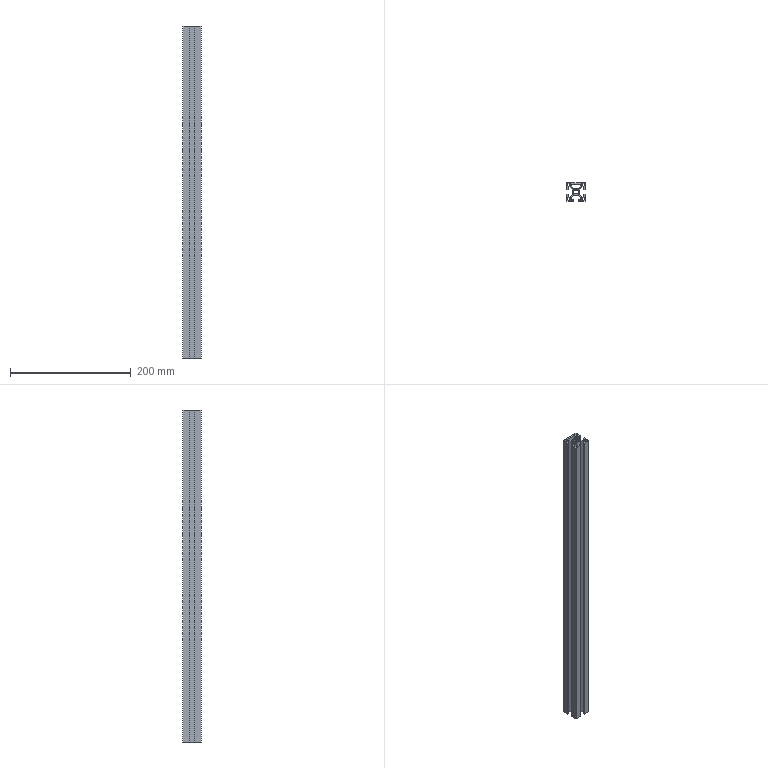Part | STEP file | 602-13-0039 | 1 solid | 75 faces | box 30 x 30 x 550 mm | volume 186584 mm3 | plane 66 | cylinder 9 | commonest cylinder face diameters 7.6 x5 12 x4